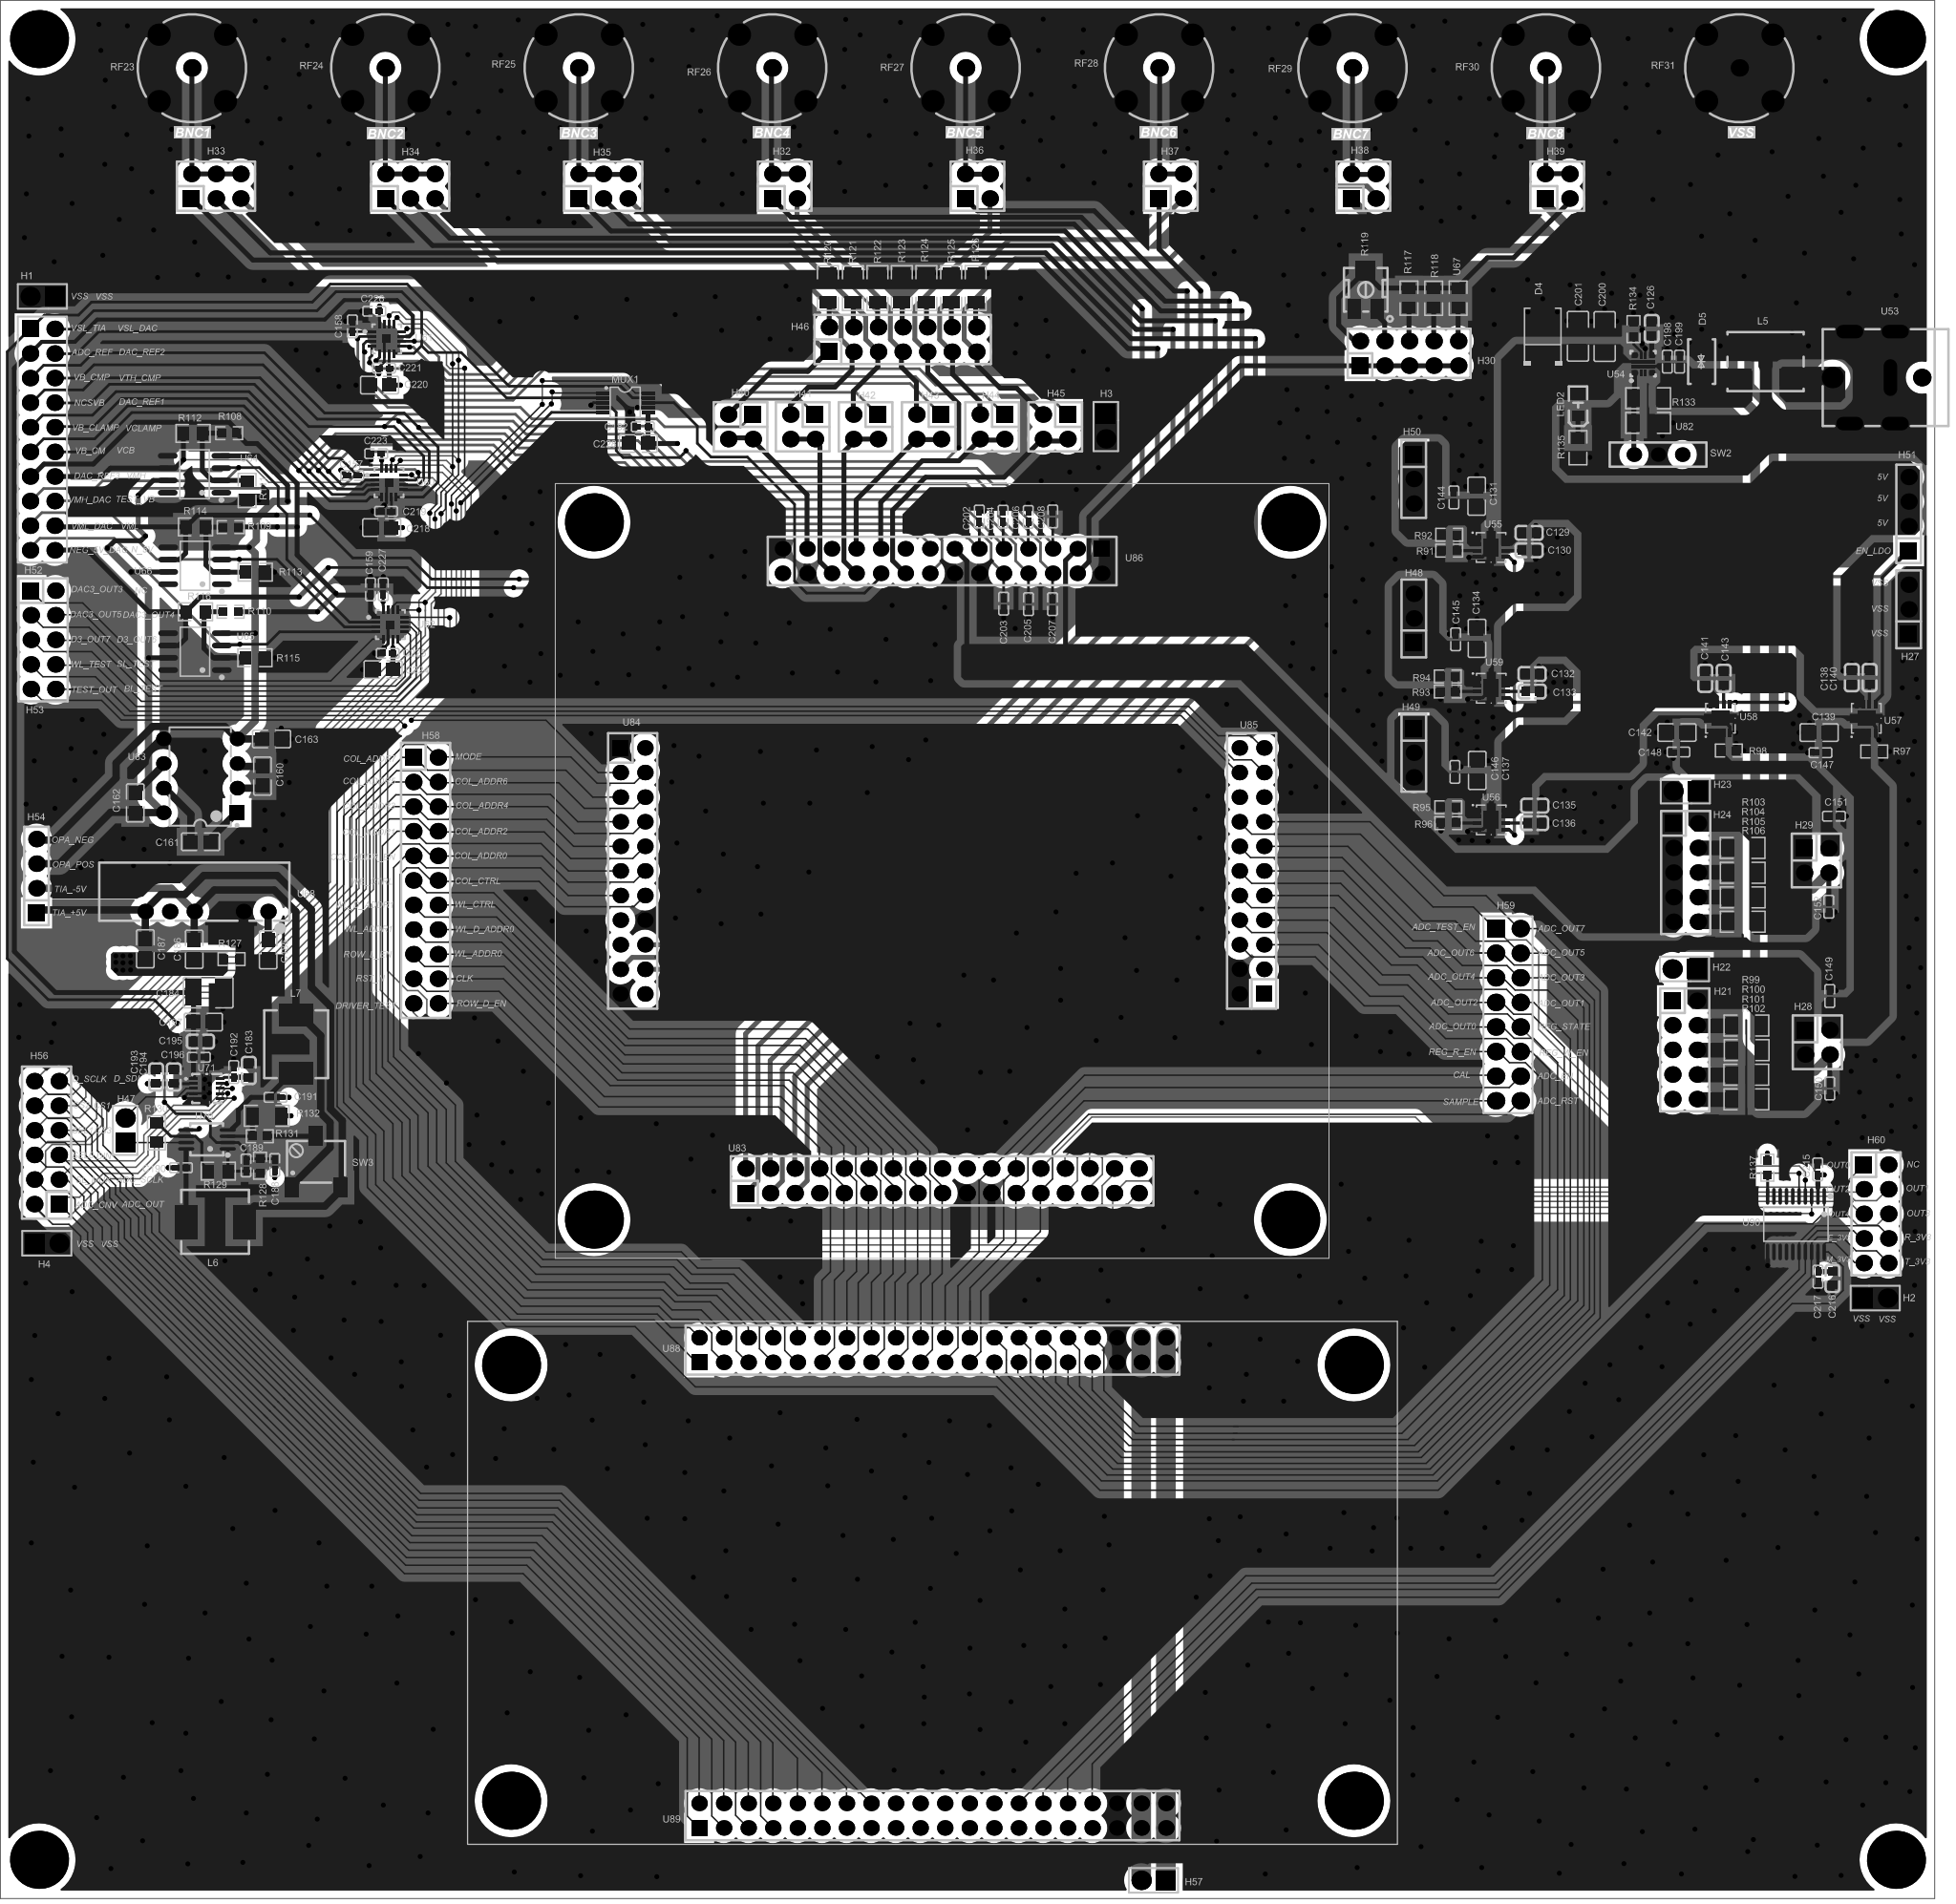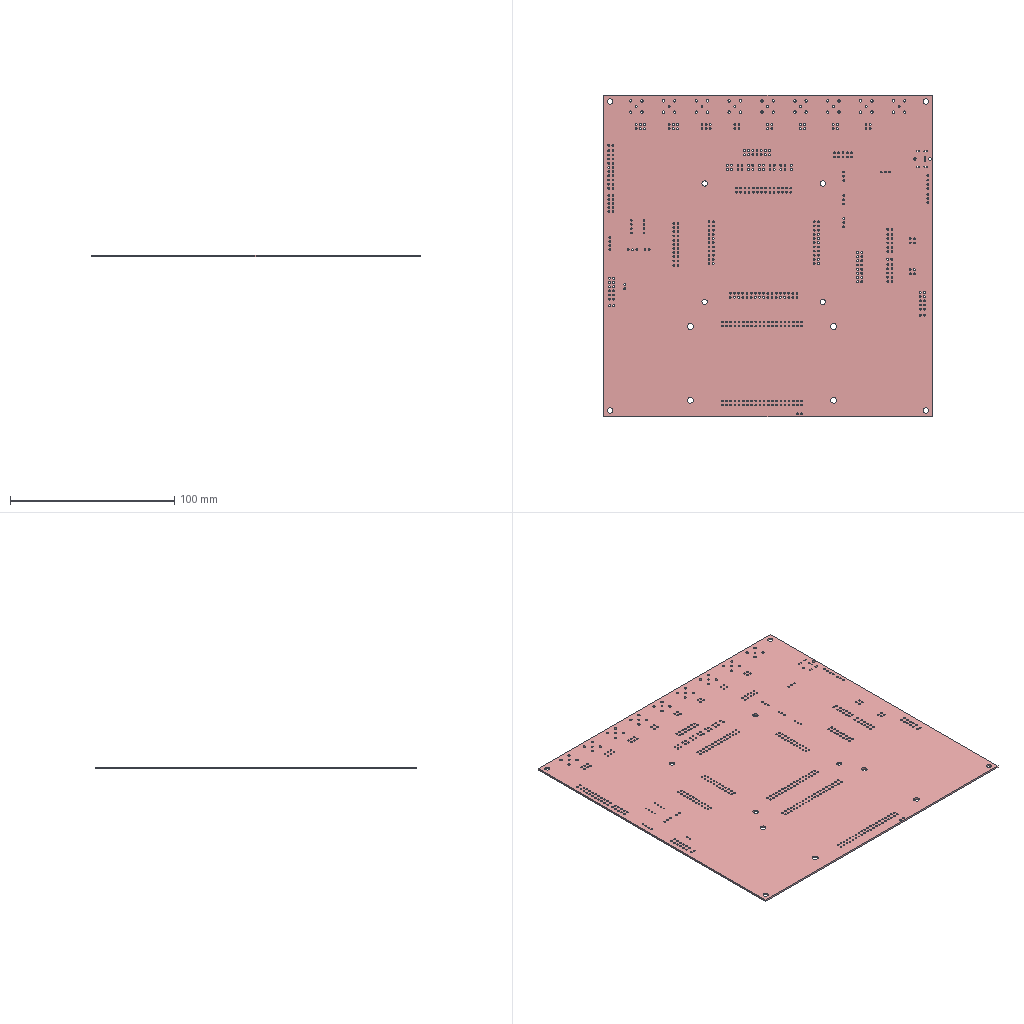Circuit board layout | Altium Designer | box 200 x 196 x 1.1 mm
Layer stack:
# Altium Designer layer stack of  (unit mm; dielectric type: 0 none, 1 core, 2 prepreg, 3 surface material)
index,name,kind,layer,copper_thickness_mm,dielectric_type,dielectric_thickness_mm,dielectric_material,dielectric_constant
0,Top Paste Mask Layer,other,,,,,,
1,Top Silkscreen Layer,other,,,,,,
2,Top Solder Mask Layer,dielectric,,,3,0.0102,Solder Resist,3.5
3,Top Layer,copper,Top Layer,0.0356,,,,
4,Dielectric1,dielectric,,,1,0.32,FR-4,4.8
5,GND,copper,GND,0.0356,,,,
6,Dielectric5,dielectric,,,2,0.32,FR-4,4.8
7,VCC,copper,VCC,0.0356,,,,
8,Dielectric6,dielectric,,,1,0.32,FR-4,4.8
9,Bottom Layer,copper,Bottom Layer,0.0356,,,,
10,Bottom Solder Mask Layer,dielectric,,,3,0.0102,Solder Resist,3.5
11,Bottom Silkscreen Layer,other,,,,,,
12,Bottom Paste Mask Layer,other,,,,,,
# drill layer pairs: low layer,high layer
drill_pair,Top Layer,Bottom Layer
Part placement:
Designator,Comment,Layer,Footprint,Center-X(mm),Center-Y(mm),Rotation
U59,#NAME?,TopLayer,VSON-8_L3.0-W3.0-P0.65-TL-EP,154.151,124.968,360
U58,#NAME?,TopLayer,VSON-8_L3.0-W3.0-P0.65-TL-EP,177.848,121.874,90
U57,#NAME?,TopLayer,VSON-8_L3.0-W3.0-P0.65-TL-EP,192.929,121.867,90
U56,#NAME?,TopLayer,VSON-8_L3.0-W3.0-P0.65-TL-EP,154.151,111.379,360
U55,#NAME?,TopLayer,VSON-8_L3.0-W3.0-P0.65-TL-EP,154.129,139.509,360
U70,#NAME?,TopLayer,MSOP-8_L3.0-W3.0-P0.65-LS5.0-TL,21.361,78.386,180
H60,#NAME?,TopLayer,HDR-TH_10P-P2.54-V-M-R2-C5-S2.54,193.938,70.7,270
H59,#NAME?,TopLayer,HDR-TH_16P-P2.54-V-M-R2-C8-S2.54,155.88,91.262,270
H58,#NAME?,TopLayer,HDR-TH_22P-P2.54-V-M-R2-C11-S2.54,43.967,105.131,270
H57,#NAME?,TopLayer,HDR-TH_2P-P2.54-V-M,119.228,1.88,180
C217,100nF,TopLayer,C0402,187.935,64.211,90
C216,1uF,TopLayer,C0603,189.433,64.033,90
C215,100nF,TopLayer,C0402,187.909,75.286,270
R137,10kO,TopLayer,R0603,182.702,75.463,270
U90,#NAME?,TopLayer,TSSOP-20_L6.5-W4.4-P0.65-LS6.4-BL,185.652,69.639,180
U89,#NAME?,TopLayer,HDR-TH_40P-P2.54-V-F-R2-C20-S2.54,96.378,8.56,360
U88,#NAME?,TopLayer,HDR-TH_40P-P2.54-V-F-R2-C20-S2.54,96.378,56.64,360
C208,100nF,TopLayer,C0402,108.814,142.709,90
C207,100nF,TopLayer,C0402,108.788,133.655,270
C206,100nF,TopLayer,C0402,106.274,142.658,90
C205,100nF,TopLayer,C0402,106.299,133.655,270
C204,100nF,TopLayer,C0402,103.683,142.684,90
C203,100nF,TopLayer,C0402,103.734,133.706,270
C202,100nF,TopLayer,C0402,101.219,142.697,90
U86,#NAME?,TopLayer,HDR-TH_28P-P2.54-V-F-R2-C14-S2.54-1,97.375,138.108,180
U85,#NAME?,TopLayer,HDR-TH_22P-P2.54-V-F-R2-C11-S2.54,129.375,106.108,90
U84,#NAME?,TopLayer,HDR-TH_22P-P2.54-V-F-R2-C11-S2.54,65.375,106.108,270
U83,#NAME?,TopLayer,HDR-TH_34P-P2.54-V-F-R2-C17-S2.54-1,97.375,74.108,360
C228,10uF,TopLayer,C0805,65.964,150.241,360
C227,100nF,TopLayer,C0402,39.592,135.179,270
C226,100nF,TopLayer,C0402,38.659,163.906,360
C225,100nF,TopLayer,C0402,40.049,128.575,360
C224,10uF,TopLayer,C0805,39.573,126.898,360
C223,100nF,TopLayer,C0402,38.862,149.2,360
C221,100nF,TopLayer,C0402,39.667,158.025,360
C220,10uF,TopLayer,C0805,39.21,156.272,360
C219,100nF,TopLayer,C0402,39.886,143.236,360
C218,10uF,TopLayer,C0805,39.429,141.56,360
H56,#NAME?,TopLayer,HDR-TH_12P-P2.54-V-M-R2-C6-S2.54,4.775,78.054,90
H54,#NAME?,TopLayer,HDR-TH_4P-P2.54-V-M,3.734,105.588,90
H53,#NAME?,TopLayer,HDR-TH_10P-P2.54-V-M-R2-C5-S2.54,4.42,129.972,270
H52,#NAME?,TopLayer,HDR-TH_20P-P2.54-V-M-R2-C10-S2.54,4.343,150.647,270
C197,10uF,TopLayer,C0805,20.98,90.501,180
C196,100nF,TopLayer,C0402,20.523,86.869,360
C195,1nF,TopLayer,C0603,20.675,88.495,180
C194,1nF,TopLayer,C0603,17.932,84.837,90
C193,1uF,TopLayer,C0603,16.103,84.837,90
C192,100nF,TopLayer,C0402,24.13,85.344,90
H47,#NAME?,TopLayer,HDR-TH_2P-P2.54-V-M,12.903,79.324,90
L7,10uH,TopLayer,IND-SMD_L7.3-W6.8,30.582,88.214,270
C191,100nF,TopLayer,C0402,28.448,82.728,180
R132,100O,TopLayer,R1206,27.534,80.823,180
R131,100kO,TopLayer,R0603,26.822,78.715,180
SW3,50kO,TopLayer,RES-ADJ-SMD_3P-L6.0-W4.3-P5.00-BL,32.639,76.073,360
R130,1kO,TopLayer,R0805,16.129,79.071,270
R129,1kO,TopLayer,R0805,22.53,75.109,180
L6,10uH,TopLayer,IND-SMD_L7.3-W6.8,22.199,69.877,360
C190,100nF,TopLayer,C0402,18.669,75.463,180
R128,10kO,TopLayer,R0603,26.848,75.668,270
C189,24pF,TopLayer,C0402,25.4,75.693,90
C188,68pF,TopLayer,C0402,28.372,75.744,270
R127,0O,TopLayer,R0603,23.901,97.003,360
C187,4.7uF,TopLayer,C0805,14.986,98.069,270
C186,4.7uF,TopLayer,C0805,20.041,98.019,270
C185,4.7uF,TopLayer,C0805,27.686,97.968,270
C184,100uF,TopLayer,C1210,21.488,93.549,180
C183,1uF,TopLayer,C0603,25.679,85.496,270
R126,1MO,TopLayer,R1206,100.838,166.294,90
R125,1MO,TopLayer,R1206,98.311,166.294,90
R124,1MO,TopLayer,R1206,95.746,166.294,90
R123,1MO,TopLayer,R1206,93.206,166.294,90
R122,1MO,TopLayer,R1206,90.691,166.294,90
R121,1MO,TopLayer,R1206,88.151,166.294,90
R120,1MO,TopLayer,R1206,85.561,166.294,90
H46,#NAME?,TopLayer,HDR-TH_14P-P2.54-V-M-R2-C7-S2.54,93.294,160.985,360
H45,#NAME?,TopLayer,HDR-TH_4P-P2.54-V-M-R2-C2-S2.54,109.068,151.968,180
H44,#NAME?,TopLayer,HDR-TH_4P-P2.54-V-M-R2-C2-S2.54,102.54,151.968,180
H43,#NAME?,TopLayer,HDR-TH_4P-P2.54-V-M-R2-C2-S2.54,95.987,151.968,180
H42,#NAME?,TopLayer,HDR-TH_4P-P2.54-V-M-R2-C2-S2.54,89.459,151.968,180
H41,#NAME?,TopLayer,HDR-TH_4P-P2.54-V-M-R2-C2-S2.54,82.956,151.968,180
H40,#NAME?,TopLayer,HDR-TH_4P-P2.54-V-M-R2-C2-S2.54,76.53,151.968,180
C182,100nF,TopLayer,C0402,66.421,151.968,360
MUX1,#NAME?,TopLayer,VSSOP-10_L3.0-W3.0-P0.50-LS4.9-BL,64.618,154.459,270
RF31,#NAME?,TopLayer,ANT-TH_DOSIN-801-0057,179.803,189.027,0
RF30,#NAME?,TopLayer,ANT-TH_DOSIN-801-0057,159.803,189.027,0
RF29,#NAME?,TopLayer,ANT-TH_DOSIN-801-0057,139.803,189.027,0
RF28,#NAME?,TopLayer,ANT-TH_DOSIN-801-0057,119.803,189.027,0
RF27,#NAME?,TopLayer,ANT-TH_DOSIN-801-0057,99.803,189.027,0
RF26,#NAME?,TopLayer,ANT-TH_DOSIN-801-0057,79.803,189.027,0
RF25,#NAME?,TopLayer,ANT-TH_DOSIN-801-0057,59.803,189.027,0
RF24,#NAME?,TopLayer,ANT-TH_DOSIN-801-0057,39.803,189.027,0
H39,#NAME?,TopLayer,HDR-TH_4P-P2.54-V-M-R2-C2-S2.54,160.975,176.809,0
H38,#NAME?,TopLayer,HDR-TH_4P-P2.54-V-M-R2-C2-S2.54,140.932,176.809,0
H37,#NAME?,TopLayer,HDR-TH_4P-P2.54-V-M-R2-C2-S2.54,121.011,176.809,0
H36,#NAME?,TopLayer,HDR-TH_4P-P2.54-V-M-R2-C2-S2.54,101.026,176.809,0
H35,#NAME?,TopLayer,HDR-TH_6P-P2.54-V-M-R2-C3-S2.54,62.327,176.809,0
H34,#NAME?,TopLayer,HDR-TH_6P-P2.54-V-M-R2-C3-S2.54,42.367,176.809,0
H33,#NAME?,TopLayer,HDR-TH_6P-P2.54-V-M-R2-C3-S2.54,22.292,176.809,0
H32,#NAME?,TopLayer,HDR-TH_4P-P2.54-V-M-R2-C2-S2.54,81.092,176.809,0
RF23,#NAME?,TopLayer,ANT-TH_DOSIN-801-0057,19.803,189.027,0
U71,#NAME?,TopLayer,VSON-10_L3.0-W3.0-P0.50-TL-EP-3,21.341,83.643,360
U68,#NAME?,TopLayer,PWRM-TH_A05XXS-1WR3,21.324,101.917,180
R119,200kO,TopLayer,RES-ADJ-SMD_3P-L4.5-W4.5-P2.30-BL-FS,141.173,166.116,90
U67,8kO,TopLayer,R0805,150.724,165.252,90
R118,5kO,TopLayer,R0805,148.199,165.242,90
R117,4kO,TopLayer,R0805,145.644,165.252,90
H30,#NAME?,TopLayer,HDR-TH_10P-P2.54-V-M-R2-C5-S2.54,145.659,159.553,360
C163,4.7uF,TopLayer,C0805,28.042,119.736,180
C162,4.7uF,TopLayer,C0805,13.945,113.132,270
C161,4.7uF,TopLayer,C0805,20.701,109.118,360
C160,4.7uF,TopLayer,C0805,27.102,115.9,270
R116,20kO,TopLayer,R0805,20.171,132.869,180
R115,20kO,TopLayer,R0805,26.317,128.119,180
R114,20kO,TopLayer,R0805,20.178,141.632,180
R113,20kO,TopLayer,R0805,26.35,136.959,180
R112,20kO,TopLayer,R0805,19.924,151.284,180
R111,20kO,TopLayer,R0805,25.512,145.391,90
U66,#NAME?,TopLayer,SOIC-8_L4.9-W3.9-P1.27-LS6.0-BL,20.127,137.619,90
U65,#NAME?,TopLayer,SOIC-8_L4.9-W3.9-P1.27-LS6.0-BL,20.121,128.749,90
U64,#NAME?,TopLayer,SOIC-8_L4.9-W3.9-P1.27-LS6.0-BL,20.076,147.068,90
U63,#NAME?,TopLayer,DIP-8_L10.1-W6.3-P2.54-LS7.6-BL,20.66,115.927,90
R110,10kO,TopLayer,R0603,23.803,132.869,180
R109,10kO,TopLayer,R0603,23.81,141.607,180
R108,10kO,TopLayer,R0603,23.657,151.31,180
C159,150nF,TopLayer,C0402,38.271,135.179,270
C158,150nF,TopLayer,C0402,36.398,162.331,270
C157,150nF,TopLayer,C0402,36.381,146.945,360
U62,#NAME?,TopLayer,WQFN-16_L3.0-W3.0-P0.50-TL-EP0.8,40.329,131.547,360
U61,#NAME?,TopLayer,WQFN-16_L3.0-W3.0-P0.50-TL-EP0.8,39.946,161.047,360
U60,#NAME?,TopLayer,WQFN-16_L3.0-W3.0-P0.50-TL-EP0.8,40.186,146.209,360
R135,1kO,TopLayer,R0805,163.119,149.809,90
C201,22uF,TopLayer,C1206,163.119,161.315,270
C200,22uF,TopLayer,C1206,165.875,161.29,270
R134,681O,TopLayer,R0603,168.859,162.052,90
R133,1MO,TopLayer,R1206,170.371,154.914,180
U82,357kO,TopLayer,R1206,170.371,152.374,360
C199,100nF,TopLayer,C0402,173.622,158.699,270
C198,100nF,TopLayer,C0402,172.352,158.699,270
H51,#NAME?,TopLayer,HDR-TH_4P-P2.54-V-M,197.307,142.977,90
H50,#NAME?,TopLayer,HDR-TH_3P-P2.54-V-M,146.134,146.583,270
H49,#NAME?,TopLayer,HDR-TH_3P-P2.54-V-M,146.145,118.313,270
H48,#NAME?,TopLayer,HDR-TH_3P-P2.54-V-M,146.145,132.182,90
C152,0.1uF,TopLayer,C0402,189.052,102.413,90
C151,0.1uF,TopLayer,C0402,189.586,111.76,180
C150,0.1uF,TopLayer,C0402,189.154,83.642,90
C149,0.1uF,TopLayer,C0402,189.154,93.193,270
H29,#NAME?,TopLayer,HDR-TH_4P-P2.54-V-M-R2-C2-S2.54,187.769,107.188,270
H28,#NAME?,TopLayer,HDR-TH_4P-P2.54-V-M-R2-C2-S2.54,187.87,88.418,270
H27,#NAME?,TopLayer,HDR-TH_3P-P2.54-V-M,197.307,133.121,90
R106,100mO,TopLayer,R1206,180.149,100.864,0
R105,100O,TopLayer,R1206,180.149,103.378,0
R104,10O,TopLayer,R1206,180.149,105.918,0
R103,1O,TopLayer,R1206,180.137,108.483,0
H24,#NAME?,TopLayer,HDR-TH_10P-P2.54-V-M-R2-C5-S2.54,174.256,105.944,270
H23,#NAME?,TopLayer,HDR-TH_2P-P2.54-V-M,174.219,114.351,180
R102,100mO,TopLayer,R1206,180.53,82.525,0
R101,100O,TopLayer,R1206,180.518,85.065,0
R100,10O,TopLayer,R1206,180.555,87.605,0
R99,1O,TopLayer,R1206,180.53,90.145,0
H22,#NAME?,TopLayer,HDR-TH_2P-P2.54-V-M,174.129,95.987,180
H21,#NAME?,TopLayer,HDR-TH_10P-P2.54-V-M-R2-C5-S2.54,174.154,87.63,270
C148,0.1uF,TopLayer,C0402,173.507,118.389,360
C147,0.1uF,TopLayer,C0402,188.189,118.313,360
C146,0.1uF,TopLayer,C0402,150.393,116.332,270
C145,0.1uF,TopLayer,C0402,150.47,130.023,270
C144,0.1uF,TopLayer,C0402,150.292,144.678,270
C143,10nF,TopLayer,C0603,178.179,125.989,270
C142,4.7uF,TopLayer,C0805,173.352,120.401,360
C141,1uF,TopLayer,C0603,176.274,125.989,270
R98,10kO,TopLayer,R0603,178.714,118.542,180
C140,10nF,TopLayer,C0603,193.269,126.06,270
C139,4.7uF,TopLayer,C0805,188.053,120.394,360
C138,1uF,TopLayer,C0603,191.431,126.058,270
R97,10kO,TopLayer,R0603,193.751,118.44,180
C137,4.7uF,TopLayer,C0805,152.703,116.484,270
C136,10nF,TopLayer,C0603,158.621,111.049,180
C135,1uF,TopLayer,C0603,158.647,112.852,180
R96,10kO,TopLayer,R0603,149.706,111.049,360
R95,12.5kO,TopLayer,R0603,149.711,112.68,180
R94,30.9kO,TopLayer,R0603,149.655,126.187,360
C134,4.7uF,TopLayer,C0805,152.678,130.124,270
C133,10nF,TopLayer,C0603,158.367,124.638,180
C132,1uF,TopLayer,C0603,158.367,126.441,180
R93,10kO,TopLayer,R0603,149.655,124.638,360
C131,4.7uF,TopLayer,C0805,152.642,144.805,270
C130,10nF,TopLayer,C0603,158.056,139.217,180
C129,1uF,TopLayer,C0603,158.056,141.017,180
R92,52.3kO,TopLayer,R0603,149.809,140.818,180
R91,10kO,TopLayer,R0603,149.804,139.184,360
D5,#NAME?,TopLayer,SMA_L4.2-W2.7-LS5.0-BI,175.908,158.699,270
C126,10nF,TopLayer,C0603,170.739,162.103,270
U54,#NAME?,TopLayer,VQFN-10_L2.0-W2.0-P0.45-TL,169.863,158.445,90
SW2,#NAME?,TopLayer,SW-TH_K3-1204D,171.399,149.098,180
L5,#NAME?,TopLayer,FILTER-SMD_4P-L7.0-W6.0-TL_SMCM7060,182.512,158.699,180
D4,#NAME?,TopLayer,SMB_L4.6-W3.6-LS5.3-RD,159.475,161.468,90
LED2,LED_0805-R,TopLayer,LED_0805,163.129,154.154,90
U53,#NAME?,TopLayer,DC-IN-TH_HX-DC007B-2.5,194.047,157.048,180
H1,#NAME?,TopLayer,HDR-TH_2P-P2.54-V-M,4.343,165.43,180
H2,#NAME?,TopLayer,HDR-TH_2P-P2.54-V-M,193.853,62.001,0
H3,#NAME?,TopLayer,HDR-TH_2P-P2.54-V-M,114.3,151.994,270
H4,#NAME?,TopLayer,HDR-TH_2P-P2.54-V-M,4.801,67.666,0
Pad and via stacks, first 65 of 74 lines:
# Altium Designer via and pad stacks of  (unit mm). Each distinct definition once, with the count of objects using it.
# via: kind,start_layer,end_layer,hole_mm,diameter_mm,mode(0 simple;1 top-mid-bottom;2 full stack),diameter_per_layer,count,example_net
# pad: kind,layer,hole_mm,hole_type(0 round;1 square;2 slot),plating,top_size,top_shape(1 round;2 rect;3 octagon;9 rounded rect),mid_size,bottom_size,mode,footprint,size_per_layer,count,example
pad,Multi-Layer,3.6,0,plated,6x6,1,6x6,6x6,0,,,4,0
pad,Multi-Layer,3.2,0,plated,6x6,1,6x6,6x6,0,,,8,2
pad,Multi-Layer,1,0,plated,1.5x1.5,1,1.5x1.5,1.5x1.5,0,SW-TH_K3-1204D,,3,SW2.3
pad,Multi-Layer,1.2,0,plated,2x2,2,2x2,2x2,0,HDR-TH_2P-P2.54-V-M,,8,H4.1
pad,Multi-Layer,1.2,0,plated,2x2,1,2x2,2x2,0,HDR-TH_2P-P2.54-V-M,,8,H4.2
pad,Multi-Layer,1.1,0,plated,1.7x1.7,2,1.7x1.7,1.7x1.7,0,HDR-TH_3P-P2.54-V-M,,4,H27.1
pad,Multi-Layer,1.1,0,plated,1.7x1.7,1,1.7x1.7,1.7x1.7,0,HDR-TH_3P-P2.54-V-M,,8,H27.2
pad,Multi-Layer,1.1,0,plated,1.7x1.7,2,1.7x1.7,1.7x1.7,0,HDR-TH_4P-P2.54-V-M,,2,H51.1
pad,Multi-Layer,1.1,0,plated,1.7x1.7,1,1.7x1.7,1.7x1.7,0,HDR-TH_4P-P2.54-V-M,,6,H51.2
pad,Multi-Layer,1,0,plated,1.6x1.6,1,1.6x1.6,1.6x1.6,0,PWRM-TH_A05XXS-1WR3,,5,U68.1
pad,Multi-Layer,1.4,0,plated,2.2x2.2,1,2.2x2.2,2.2x2.2,0,DC-IN-TH_HX-DC007B-2.5,,1,U53.1
pad,Multi-Layer,0.8,2,plated,1.4x3.8,1,1.4x3.8,1.4x3.8,0,DC-IN-TH_HX-DC007B-2.5,,1,U53.2
pad,Multi-Layer,0.8,2,plated,1.4x2.8,1,1.4x2.8,1.4x2.8,0,DC-IN-TH_HX-DC007B-2.5,,4,U53.3
pad,Multi-Layer,1.8,0,unplated,1.8x1.8,1,1.8x1.8,1.8x1.8,0,DC-IN-TH_HX-DC007B-2.5,,1,U53.0
pad,Multi-Layer,0.9,0,plated,1.5x1.5,1,1.5x1.5,1.5x1.5,0,DIP-8_L10.1-W6.3-P2.54-LS7.6-BL,,7,U63.5
pad,Multi-Layer,0.9,0,plated,1.5x1.5,2,1.5x1.5,1.5x1.5,0,DIP-8_L10.1-W6.3-P2.54-LS7.6-BL,,1,U63.1
pad,Multi-Layer,1.1,0,plated,1.7x1.7,1,1.7x1.7,1.7x1.7,0,HDR-TH_10P-P2.54-V-M-R2-C5-S2.54,,45,H21.10
pad,Multi-Layer,1.1,0,plated,1.7x1.7,2,1.7x1.7,1.7x1.7,0,HDR-TH_10P-P2.54-V-M-R2-C5-S2.54,,5,H21.1
pad,Multi-Layer,1.1,0,plated,1.7x1.7,1,1.7x1.7,1.7x1.7,0,HDR-TH_12P-P2.54-V-M-R2-C6-S2.54,,11,H56.12
pad,Multi-Layer,1.1,0,plated,1.7x1.7,2,1.7x1.7,1.7x1.7,0,HDR-TH_12P-P2.54-V-M-R2-C6-S2.54,,1,H56.1
pad,Multi-Layer,1.1,0,plated,1.7x1.7,1,1.7x1.7,1.7x1.7,0,HDR-TH_14P-P2.54-V-M-R2-C7-S2.54,,13,H46.14
pad,Multi-Layer,1.1,0,plated,1.7x1.7,2,1.7x1.7,1.7x1.7,0,HDR-TH_14P-P2.54-V-M-R2-C7-S2.54,,1,H46.1
pad,Multi-Layer,1.2,0,plated,1.8x1.8,1,1.8x1.8,1.8x1.8,0,HDR-TH_16P-P2.54-V-M-R2-C8-S2.54,,15,H59.16
pad,Multi-Layer,1.2,0,plated,1.8x1.8,2,1.8x1.8,1.8x1.8,0,HDR-TH_16P-P2.54-V-M-R2-C8-S2.54,,1,H59.1
pad,Multi-Layer,1.1,0,plated,1.7x1.7,1,1.7x1.7,1.7x1.7,0,HDR-TH_20P-P2.54-V-M-R2-C10-S2.54,,19,H52.20
pad,Multi-Layer,1.1,0,plated,1.7x1.7,2,1.7x1.7,1.7x1.7,0,HDR-TH_20P-P2.54-V-M-R2-C10-S2.54,,1,H52.1
pad,Multi-Layer,1.05,0,plated,1.6x1.6,2,1.6x1.6,1.6x1.6,0,HDR-TH_22P-P2.54-V-F-R2-C11-S2.54,,2,U84.1
pad,Multi-Layer,1.05,0,plated,1.6x1.6,1,1.6x1.6,1.6x1.6,0,HDR-TH_22P-P2.54-V-F-R2-C11-S2.54,,42,U84.2
pad,Multi-Layer,1.1,0,plated,1.7x1.7,2,1.7x1.7,1.7x1.7,0,HDR-TH_22P-P2.54-V-M-R2-C11-S2.54,,1,H58.1
pad,Multi-Layer,1.1,0,plated,1.7x1.7,1,1.7x1.7,1.7x1.7,0,HDR-TH_22P-P2.54-V-M-R2-C11-S2.54,,21,H58.2
pad,Multi-Layer,1.02,0,plated,1.6x1.6,1,1.6x1.6,1.6x1.6,0,HDR-TH_28P-P2.54-V-F-R2-C14-S2.54-1,,27,U86.28
pad,Multi-Layer,1.02,0,plated,1.6x1.6,2,1.6x1.6,1.6x1.6,0,HDR-TH_28P-P2.54-V-F-R2-C14-S2.54-1,,1,U86.1
pad,Multi-Layer,1.1,0,plated,1.7x1.7,2,1.7x1.7,1.7x1.7,0,HDR-TH_34P-P2.54-V-F-R2-C17-S2.54-1,,1,U83.1
pad,Multi-Layer,1.1,0,plated,1.7x1.7,1,1.7x1.7,1.7x1.7,0,HDR-TH_34P-P2.54-V-F-R2-C17-S2.54-1,,33,U83.34
pad,Multi-Layer,1,0,plated,1.6x1.6,1,1.6x1.6,1.6x1.6,0,HDR-TH_40P-P2.54-V-F-R2-C20-S2.54,,78,U88.40
pad,Multi-Layer,1,0,plated,1.6x1.6,2,1.6x1.6,1.6x1.6,0,HDR-TH_40P-P2.54-V-F-R2-C20-S2.54,,2,U88.1
pad,Multi-Layer,1.1,0,plated,1.7x1.7,2,1.7x1.7,1.7x1.7,0,HDR-TH_4P-P2.54-V-M-R2-C2-S2.54,,13,H28.1
pad,Multi-Layer,1.1,0,plated,1.7x1.7,1,1.7x1.7,1.7x1.7,0,HDR-TH_4P-P2.54-V-M-R2-C2-S2.54,,39,H28.2
pad,Multi-Layer,1.1,0,plated,1.7x1.7,1,1.7x1.7,1.7x1.7,0,HDR-TH_6P-P2.54-V-M-R2-C3-S2.54,,15,H33.6
pad,Multi-Layer,1.1,0,plated,1.7x1.7,2,1.7x1.7,1.7x1.7,0,HDR-TH_6P-P2.54-V-M-R2-C3-S2.54,,3,H33.1
pad,Multi-Layer,1.5,0,plated,2.3x2.3,1,2.3x2.3,2.3x2.3,0,ANT-TH_DOSIN-801-0057,,36,RF23.5
pad,Multi-Layer,1.1,0,plated,1.8x1.8,1,1.8x1.8,1.8x1.8,0,ANT-TH_DOSIN-801-0057,,9,RF23.1
pad,Top Layer,0,0,plated,2x2,2,2x2,2x2,0,RES-ADJ-SMD_3P-L4.5-W4.5-P2.30-BL-FS,,1,R119.2
pad,Top Layer,0,0,plated,2x1.3,2,2x1.3,2x1.3,0,RES-ADJ-SMD_3P-L4.5-W4.5-P2.30-BL-FS,,2,R119.1
pad,Top Layer,0,0,plated,1.208x1.701,2,1.208x1.701,1.208x1.701,0,R1206,,36,R132.1
pad,Top Layer,0,0,plated,0.7901x0.54,2,0.7901x0.54,0.7901x0.54,0,C0402,,72,C198.2
pad,Top Layer,0,0,plated,0.8x0.9,2,0.8x0.9,0.8x0.9,0,C0603,,32,C126.2
pad,Top Layer,0,0,plated,1.41x1.35,2,1.41x1.35,1.41x1.35,0,C0805,,34,C160.2
pad,Top Layer,0,0,plated,1.485x1.728,2,1.485x1.728,1.485x1.728,0,C1206,,4,C200.2
pad,Top Layer,0,0,plated,1.635x2.7,2,1.635x2.7,1.635x2.7,0,C1210,,2,C184.1
pad,Top Layer,0,0,plated,0.8065x0.864,2,0.8065x0.864,0.8065x0.864,0,R0603,,32,R91.2
pad,Top Layer,0,0,plated,1.133x1.377,2,1.133x1.377,1.133x1.377,0,R0805,,24,R135.2
pad,Top Layer,0,0,plated,1x1.25,2,1x1.25,1x1.25,0,LED_0805,,2,LED2.2
pad,Top Layer,0,0,plated,2.35x3.5,2,2.35x3.5,2.35x3.5,0,IND-SMD_L7.3-W6.8,,4,L6.2
pad,Top Layer,0,0,plated,2x1.8,2,2x1.8,2x1.8,0,SMA_L4.2-W2.7-LS5.0-BI,,2,D5.1
pad,Top Layer,0,0,plated,2.047x2.192,2,2.047x2.192,2.047x2.192,0,SMB_L4.6-W3.6-LS5.3-RD,,2,D4.2
pad,Top Layer,0,0,plated,0.6x0.6,1,0.6x0.6,0.6x0.6,0,VQFN-10_L2.0-W2.0-P0.45-TL,,4,U54.1
pad,Top Layer,0,0,plated,0.3x2.4,2,0.3x2.4,0.3x2.4,0,VQFN-10_L2.0-W2.0-P0.45-TL,,2,U54.5
pad,Top Layer,0,0,plated,0.25x0.6,2,0.25x0.6,0.25x0.6,0,VQFN-10_L2.0-W2.0-P0.45-TL,,4,U54.2
pad,Top Layer,0,0,plated,1.52x1.78,2,1.52x1.78,1.52x1.78,0,VSON-8_L3.0-W3.0-P0.65-TL-EP,,5,U55.9
pad,Top Layer,0,0,plated,0.34x0.8499,2,0.34x0.8499,0.34x0.8499,0,VSON-8_L3.0-W3.0-P0.65-TL-EP,,40,U55.8
pad,Top Layer,0,0,plated,2.5x1.75,2,2.5x1.75,2.5x1.75,0,FILTER-SMD_4P-L7.0-W6.0-TL_SMCM7060,,4,L5.4
Copper pours:
name,layer,net,type(0 solid;1 hatched;2 none)
Bottom Layer-No Net,Top Layer,AVDD,0
Bottom Layer-No Net,Top Layer,1P8V,0
Bottom Layer-No Net,Top Layer,DAC_VDD,0
Bottom Layer-No Net,Top Layer,3P3V,0
Bottom Layer-No Net,Top Layer,LDO_DVDD,0
Bottom Layer-No Net,Top Layer,LDO_AVDD,0
Bottom Layer-No Net,Top Layer,NetC198_2,0
Bottom Layer-No Net,Top Layer,5V,0
Bottom Layer-No Net,Top Layer,NetL5_1,0
Bottom Layer-No Net,Top Layer,TP_AVDD,0
Bottom Layer-No Net,Top Layer,TP_DVDD,0
Bottom Layer-No Net,Top Layer,0V,0
Bottom Layer-No Net,Top Layer,VSS,0
Bottom Layer-No Net,Bottom Layer,VSS,0
Design rules, without the lines most boards share:
# Altium Designer design rules of  (exported by Altium Designer, unit mm)
# columns: name | kind | enabled | priority | scope1 | scope2 | descriptor | typed fields (field=value)
Clearance | 0 | enabled | 2 | All | All | Clearance Constraint (Gap=6mil) (All),(All) | gap=0.1524
PlaneConnect | 6 | enabled | 1 | All | All | Power Plane Connect Rule(Direct Connect )(Expansion=20mil) (Conductor Width=10mil) (Air Gap=10mil) (Entries=4) (All) | relief_conductor_width=0.254 relief_entries=4 relief_expansion=0.508
PlaneClearance | 12 | enabled | 1 | All | All | Power Plane Clearance (Clearance =6mil) (All) | clearance=0.1524
PolygonConnect | 20 | enabled | 1 | All | All | Polygon Connect Rule(Direct Connect )(Conductor Width=10mil) (Relief Angle=90 Angle) (Entries=4) (Air Gap Width=10mil) (All),(All) | connect_style(0=relief,1=direct,2=none)=1 relief_conductor_width=0.254 relief_entries=4
Width | 2 | enabled | 1 | All | All | Width Constraint (Min=6mil) (Max=120mil) (Preferred=6mil) (All) |
RoutingVias | 11 | enabled | 1 | All | All | Routing Via (MinHoleWidth=12mil) (MaxHoleWidth=12mil) (PreferredHoleWidth=12mil) (MinWidth=20mil) (MaxWidth=20mil) (PreferedWidth=20mil) (All) | via_min_hole=0.3048 via_max_hole=0.3048 via_preferred_diameter=0.508 via_preferred_hole=0.3048
SolderMaskExpansion | 13 | enabled | 1 | All | All | Solder Mask Expansion (Expansion =4mil) (All) | expansion=0.1016
HoleSize | 42 | enabled | 1 | All | All | Hole Size Constraint (Min=1mil) (Max=500mil) (All) |
DiffPairsRouting | 51 | enabled | 1 | All | All | Differential Pairs Uncoupled Length using the Gap Constraints (Min=6mil) (Max=6mil) (Prefered=6mil)  and Width Constraints (Min=15mil) (Max=15mil) (Prefered=15mil) (All) |
HoleToHoleClearance | 52 | enabled | 1 | All | All | Hole To Hole Clearance (Gap=0mil) (All),(All) | gap=0
MinimumSolderMaskSliver | 53 | enabled | 1 | All | All | Minimum Solder Mask Sliver (Gap=0mil) (All),(All) |
SilkToSolderMaskClearance | 54 | enabled | 1 | IsPad | All | Silk To Solder Mask (Clearance=0mil) (IsPad),(All) |
SilkToSilkClearance | 55 | enabled | 1 | All | All | Silk to Silk (Clearance=0mil) (All),(All) |
Clearance_1 | 0 | enabled | 1 | inpolygon | All | Clearance Constraint (Gap=6mil) (inpolygon),(All) | gap=0.1524
Classes set for this board:
# Altium Designer classes of  (member kind: 0 net, 1 component, 2 from-to, 3 pad, 4 layer, 5 differential pair, 6 design channel, 7 polygon, 8 structure, 9 xSignal)
# columns: class name | member kind | superclass | members
4_Digital.schdoc | 1 | no | C215; C216; C217; H57; H58; H59; H60; R137; U88; U89; U90;
3_ISC_Chip.schdoc | 1 | no | C202; C203; C204; C205; C206; C207; C208; U83; U84; U85; U86;
2_ADC_DAC.schdoc | 1 | no | C157; C158; C159; C160; C161; C162; C163; C182; C183; C184; C185; C186; C187; C188; C189; C190; C191; C192; C193; C194; C195; C196; C197; C218; C219; C220; C221; C223; C224; C225; C226; C227; C228; H30; H32; H33; H34; H35; H36; H37; H38; H39; H40; H41; H42; H43; H44; H45; H46; H47; H52; H53; H54; H56; L6; L7; MUX1; R108; R109; R110; R111; R112; R113; R114; R115; R116; R117; R118; R119; R120; R121; R122; R123; R124; R125; R126; R127; R128; R129; R130; R131; R132; RF23; RF24; RF25; RF26; RF27; RF28; RF29; RF30; RF31; SW3; U60; U61; U62; U63; U64; U65; U66; U67; U68; U70; U71;
1_Power.schdoc | 1 | no | C126; C129; C130; C131; C132; C133; C134; C135; C136; C137; C138; C139; C140; C141; C142; C143; C144; C145; C146; C147; C148; C149; C150; C151; C152; C198; C199; C200; C201; D4; D5; H21; H22; H23; H24; H27; H28; H29; H48; H49; H50; H51; L5; LED2; R91; R92; R93; R94; R95; R96; R97; R98; R99; R100; R101; R102; R103; R104; R105; R106; R133; R134; R135; SW2; U53; U54; U55; U56; U57; U58; U59; U82; U55; U56; U57; U58; U59; H1; H2; H3; H4;